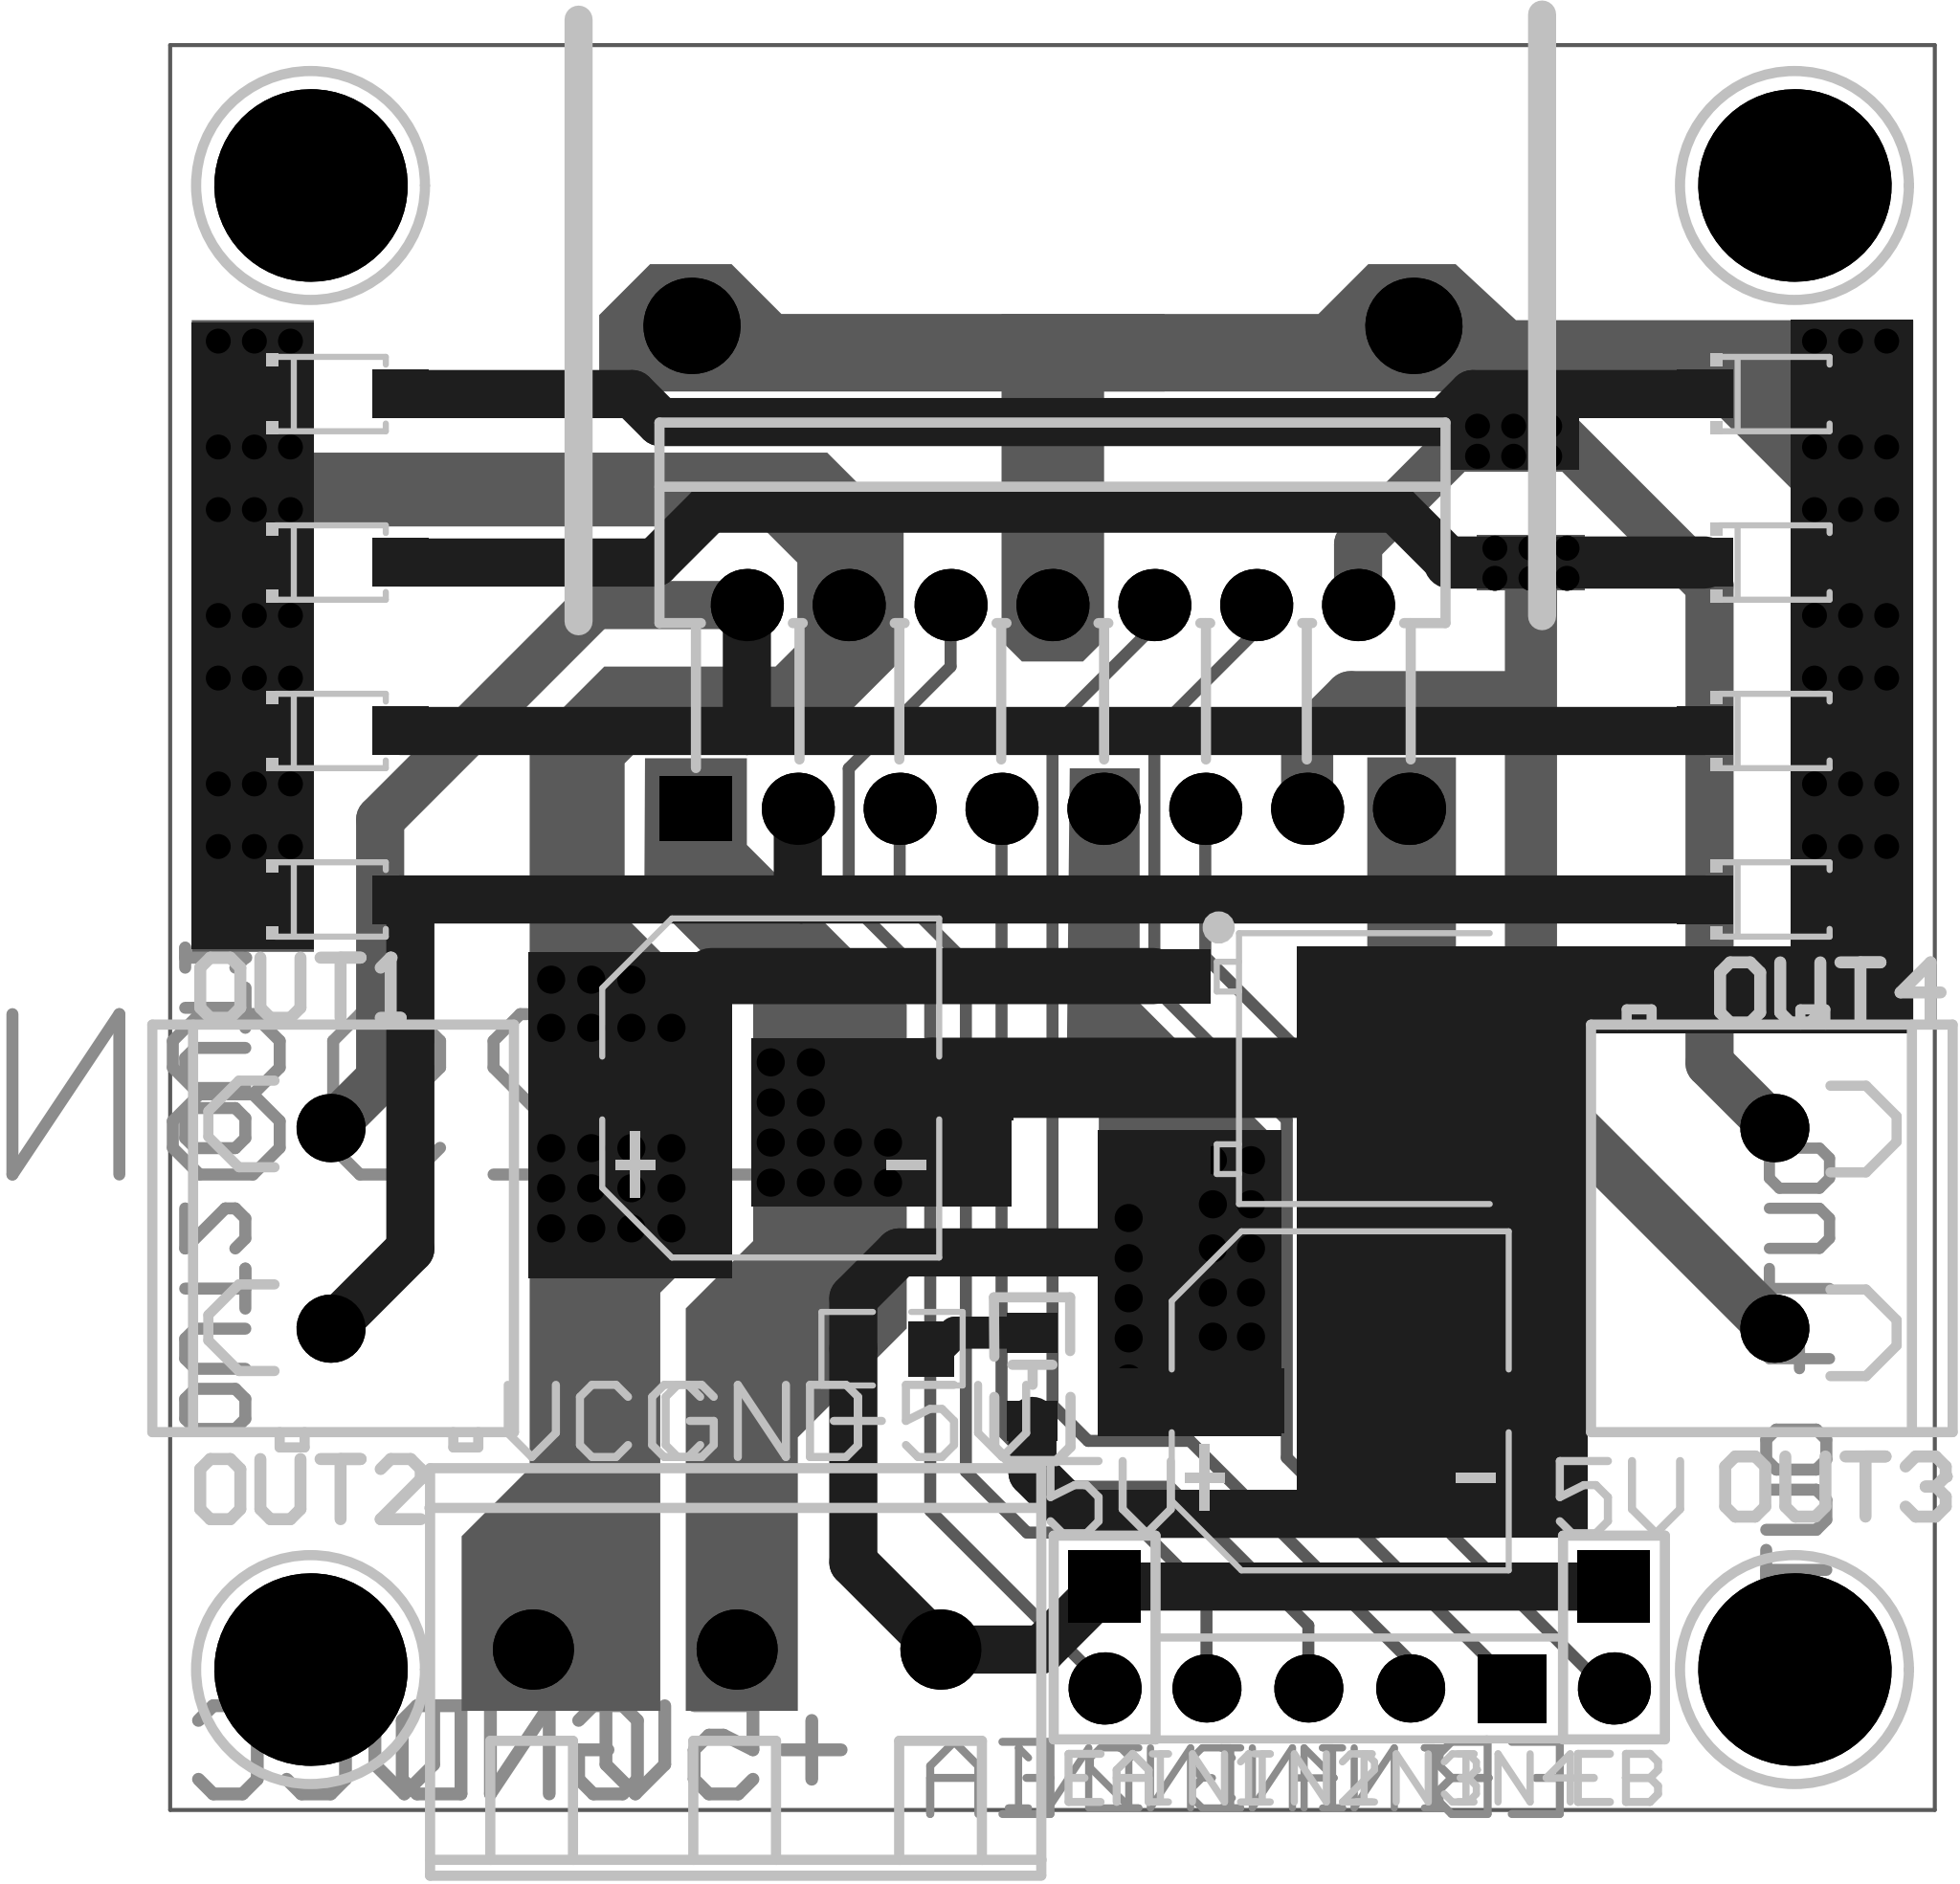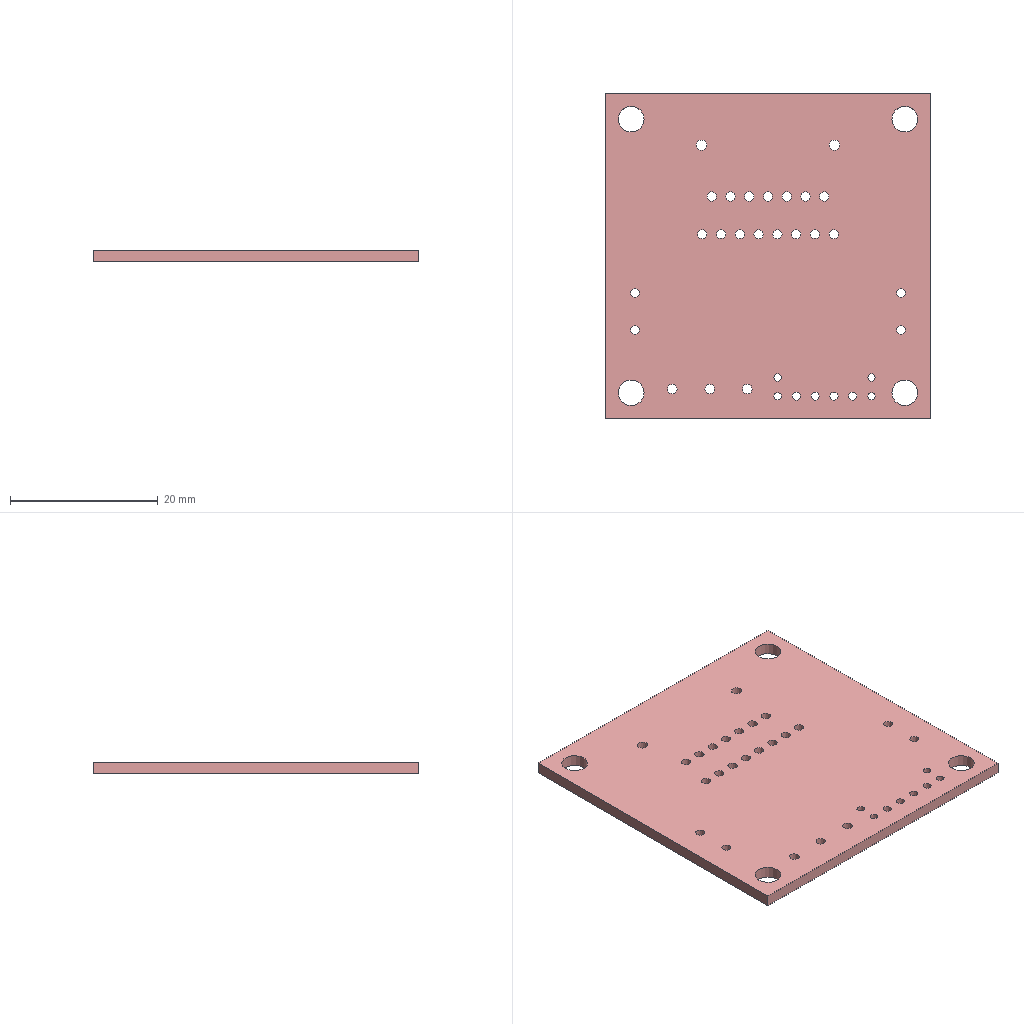Circuit board layout | Altium Designer | box 44 x 44 x 1.6 mm
Layer stack:
# Altium Designer layer stack of  (unit mm; dielectric type: 0 none, 1 core, 2 prepreg, 3 surface material)
index,name,kind,layer,copper_thickness_mm,dielectric_type,dielectric_thickness_mm,dielectric_material,dielectric_constant
0,Top Paste Mask Layer,other,,,,,,
1,Top Silkscreen Layer,other,,,,,,
2,Top Solder Mask Layer,dielectric,,,3,0.01,,3.3
3,Top Layer,copper,Top Layer,0.035,,,,
4,Dielectric1,dielectric,,,3,1.51,FR4,4.5
5,Bottom Layer,copper,Bottom Layer,0.035,,,,
6,Bottom Solder Mask Layer,dielectric,,,3,0.01,,3.3
7,Bottom Silkscreen Layer,other,,,,,,
8,Bottom Paste Mask Layer,other,,,,,,
# drill layer pairs: low layer,high layer
drill_pair,Top Layer,Bottom Layer
Part placement:
Designator,Comment,Layer,Footprint,Center-X(mm),Center-Y(mm),Rotation
P1,,TopLayer,CONN-TH_3P-P5.00_WJ500V-5.08-3P,90.886,81.966,180
U2,L298N,TopLayer,multiwatt-15_l19.6-w5.0-p1.27-l,98.76,105.466,0
U8,,TopLayer,SMD_BD4.2-L4.7-W4.7-D3.0,117.26,81.466,0
H4,,TopLayer,HDR-TH_2P-P2.54-V-M-1,100.06,82.266,270
U3,,TopLayer,CONN-TH_DB302-5.0-2P,80.76,92.466,270
U4,,TopLayer,CONN-TH_DB302-5.0-2P,116.76,92.466,90
C2,,TopLayer,CAP-SMD_BD8.0-L8.3-W8.3-LS9.3-FD,105.96,88.166,0
U6,,TopLayer,SMD_BD4.2-L4.7-W4.7-D3.0,117.26,118.466,0
H3,,TopLayer,HDR-TH_2P-P2.54-V-M-1,112.76,82.266,270
LED1,,TopLayer,LED0805-RD_BLUE,98.26,88.766,90
U9,L78M05ABDT-TR,TopLayer,TO-252-2_L6.5-W6.1-P4.58-LS10.0-TL,104.76,96.466,0
D5,,TopLayer,SOD-123FL_L2.7-W1.8-LS3.8-RD,116.76,104.866,0
D6,,TopLayer,SOD-123FL_L2.7-W1.8-LS3.8-RD,116.76,100.666,0
D7,,TopLayer,SOD-123FL_L2.7-W1.8-LS3.8-RD,116.76,109.066,0
D8,,TopLayer,SOD-123FL_L2.7-W1.8-LS3.8-RD,116.76,113.266,0
C1,,TopLayer,CAP-SMD_BD8.0-L8.3-W8.3-LS9.3-FD,91.76,95.966,0
U5,,TopLayer,SMD_BD4.2-L4.7-W4.7-D3.0,80.26,118.466,0
U7,,TopLayer,SMD_BD4.2-L4.7-W4.7-D3.0,80.26,81.466,0
D4,,TopLayer,SOD-123FL_L2.7-W1.8-LS3.8-RD,80.76,113.266,0
R1,,TopLayer,R0805,94.76,89.466,180
H5,826629-4,TopLayer,HDR-TH_4P-P2.54-V-M-1,106.41,80.996,180
D1,,TopLayer,SOD-123FL_L2.7-W1.8-LS3.8-RD,80.76,104.866,0
D2,,TopLayer,SOD-123FL_L2.7-W1.8-LS3.8-RD,80.76,100.666,0
D3,,TopLayer,SOD-123FL_L2.7-W1.8-LS3.8-RD,80.76,109.066,0
Pad and via stacks:
# Altium Designer via and pad stacks of  (unit mm). Each distinct definition once, with the count of objects using it.
# via: kind,start_layer,end_layer,hole_mm,diameter_mm,mode(0 simple;1 top-mid-bottom;2 full stack),diameter_per_layer,count,example_net
# pad: kind,layer,hole_mm,hole_type(0 round;1 square;2 slot),plating,top_size,top_shape(1 round;2 rect;3 octagon;9 rounded rect),mid_size,bottom_size,mode,footprint,size_per_layer,count,example
pad,Multi-Layer,1.4,0,plated,2.4x2.4,1,2.4x2.4,2.4x2.4,0,,,2,1
pad,Multi-Layer,1.3,0,plated,1.999x1.999,1,1.999x1.999,1.999x1.999,0,CONN-TH_3P-P5.00_WJ500V-5.08-3P,,3,P1.3
pad,Multi-Layer,1.26,0,plated,1.8x1.8,1,1.8x1.8,1.8x1.8,0,multiwatt-15_l19.6-w5.0-p1.27-l,,14,U2.15
pad,Multi-Layer,1.26,0,plated,1.8x1.6,2,1.8x1.6,1.8x1.6,0,multiwatt-15_l19.6-w5.0-p1.27-l,,1,U2.1
pad,Multi-Layer,3.5,0,plated,4.8x4.8,1,4.8x4.8,4.8x4.8,0,SMD_BD4.2-L4.7-W4.7-D3.0,,4,U8.1
pad,Multi-Layer,1,0,plated,1.8x1.8,1,1.8x1.8,1.8x1.8,0,HDR-TH_2P-P2.54-V-M-1,,2,H4.2
pad,Multi-Layer,1,0,plated,1.8x1.8,2,1.8x1.8,1.8x1.8,0,HDR-TH_2P-P2.54-V-M-1,,2,H4.1
pad,Multi-Layer,1.2,0,plated,1.7x1.7,1,1.7x1.7,1.7x1.7,0,CONN-TH_DB302-5.0-2P,,4,U3.1
pad,Multi-Layer,1.1,0,plated,1.7x1.7,2,1.7x1.7,1.7x1.7,0,HDR-TH_4P-P2.54-V-M-1,,1,H5.1
pad,Multi-Layer,1.1,0,plated,1.7x1.7,1,1.7x1.7,1.7x1.7,0,HDR-TH_4P-P2.54-V-M-1,,3,H5.2
pad,Top Layer,0,0,plated,4.6x1.6,2,4.6x1.6,4.6x1.6,0,CAP-SMD_BD8.0-L8.3-W8.3-LS9.3-FD,,4,C2.1
pad,Top Layer,0,0,plated,1.001x1.25,2,1.001x1.25,1.001x1.25,0,LED0805-RD_BLUE,,2,LED1.1
pad,Top Layer,0,0,plated,6.5x6,2,6.5x6,6.5x6,0,TO-252-2_L6.5-W6.1-P4.58-LS10.0-TL,,1,U9.4
pad,Top Layer,0,0,plated,2.8x1.35,2,2.8x1.35,2.8x1.35,0,TO-252-2_L6.5-W6.1-P4.58-LS10.0-TL,,1,U9.1
pad,Top Layer,0,0,plated,2.8x1.5,2,2.8x1.5,2.8x1.5,0,TO-252-2_L6.5-W6.1-P4.58-LS10.0-TL,,1,U9.3
pad,Top Layer,0,0,plated,1.399x1.199,2,1.399x1.199,1.399x1.199,0,SOD-123FL_L2.7-W1.8-LS3.8-RD,,16,D5.2
pad,Top Layer,0,0,plated,1.133x1.377,2,1.133x1.377,1.133x1.377,0,R0805,,2,R1.2
via,Top Layer,Bottom Layer,0.381,0.7,0,,46,+5V
via,Top Layer,Bottom Layer,0.3048,0.6096,0,,12,GND
via,Top Layer,Bottom Layer,0.3404,0.62,0,,54,GND
Design rules, without the lines most boards share:
# Altium Designer design rules of  (exported by Altium Designer, unit mm)
# columns: name | kind | enabled | priority | scope1 | scope2 | descriptor | typed fields (field=value)
otherClearance | 52 | enabled | 1 | All | All | Hole To Hole Clearance (Gap=11.8mil) (All),(All) | gap=0.2997